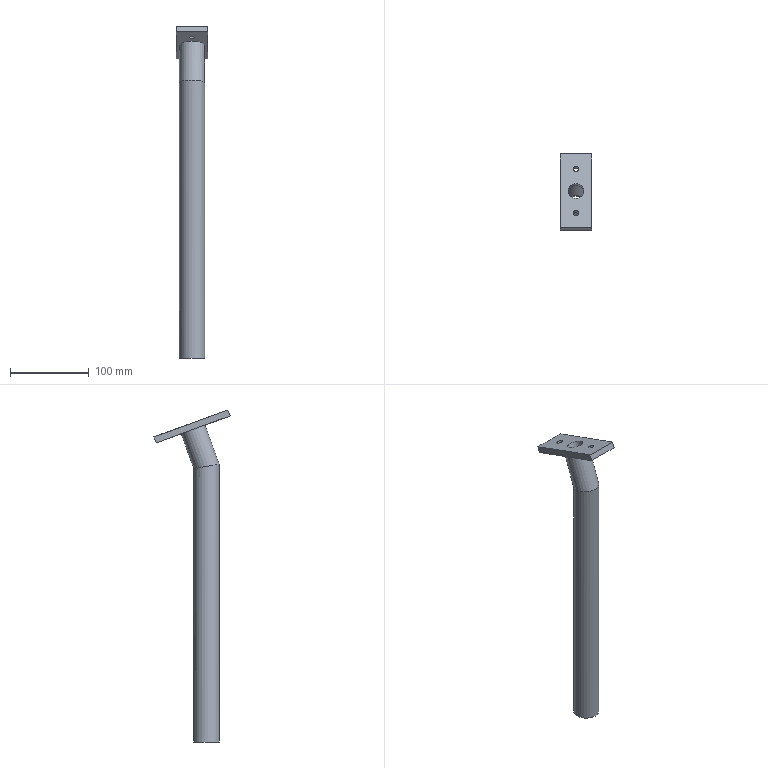Part | STEP file | 1112 | 1 solid | 15 faces | box 40 x 96.705 x 421.603 mm | volume 104269 mm3 | plane 8 | cylinder 7 | commonest cylinder face diameters 7 x2 28 x2 32 x2 20 x1
STEP:
#1=CARTESIAN_POINT('',(0.,0.,0.));
#2=DIRECTION('',(0.,0.,1.));
#3=DIRECTION('',(1.,0.,0.));
#4=AXIS2_PLACEMENT_3D('',#1,#2,#3);
#5=CARTESIAN_POINT('',(0.,-20.316,30.363));
#6=VERTEX_POINT('',#5);
#7=CARTESIAN_POINT('',(0.,11.684,24.721));
#8=VERTEX_POINT('',#7);
#9=CARTESIAN_POINT('',(0.,11.684,24.721));
#10=CARTESIAN_POINT('',(32.,11.684,24.721));
#11=CARTESIAN_POINT('',(32.,-20.316,30.363));
#12=CARTESIAN_POINT('',(0.,-20.316,30.363));
#13=CARTESIAN_POINT('',(-32.,-20.316,30.363));
#14=CARTESIAN_POINT('',(-32.,11.684,24.721));
#15=CARTESIAN_POINT('',(0.,11.684,24.721));
#16=(BOUNDED_CURVE()B_SPLINE_CURVE(3,(#9,#10,#11,#12,#13,#14,#15),.UNSPECIFIED.,.T.,.F.)B_SPLINE_CURVE_WITH_KNOTS((1,3,3,3,1),(-3.142,0.,3.142,6.283,9.425),.UNSPECIFIED.)CURVE()GEOMETRIC_REPRESENTATION_ITEM()RATIONAL_B_SPLINE_CURVE((1.,0.3333,0.3333,1.,0.3333,0.3333,1.))REPRESENTATION_ITEM(''));
#17=CARTESIAN_POINT('',(0.,-4.316,27.542));
#18=DIRECTION('',(0.,0.342,0.9397));
#19=DIRECTION('',(0.,-0.9397,0.342));
#20=AXIS2_PLACEMENT_3D('',#17,#18,#19);
#21=CYLINDRICAL_SURFACE('',#20,16.);
#22=CARTESIAN_POINT('',(9.425,2.821));
#23=CARTESIAN_POINT('',(9.364,2.821));
#24=CARTESIAN_POINT('',(9.232,2.791));
#25=CARTESIAN_POINT('',(8.995,2.593));
#26=CARTESIAN_POINT('',(8.714,2.172));
#27=CARTESIAN_POINT('',(8.392,1.474));
#28=CARTESIAN_POINT('',(8.037,0.5262));
#29=CARTESIAN_POINT('',(7.671,-0.5261));
#30=CARTESIAN_POINT('',(7.316,-1.474));
#31=CARTESIAN_POINT('',(6.994,-2.172));
#32=CARTESIAN_POINT('',(6.714,-2.593));
#33=CARTESIAN_POINT('',(6.475,-2.791));
#34=CARTESIAN_POINT('',(6.283,-2.837));
#35=CARTESIAN_POINT('',(6.092,-2.791));
#36=CARTESIAN_POINT('',(5.853,-2.593));
#37=CARTESIAN_POINT('',(5.573,-2.172));
#38=CARTESIAN_POINT('',(5.25,-1.474));
#39=CARTESIAN_POINT('',(4.896,-0.5261));
#40=CARTESIAN_POINT('',(4.529,0.5262));
#41=CARTESIAN_POINT('',(4.175,1.474));
#42=CARTESIAN_POINT('',(3.852,2.172));
#43=CARTESIAN_POINT('',(3.572,2.593));
#44=CARTESIAN_POINT('',(3.335,2.791));
#45=CARTESIAN_POINT('',(3.202,2.821));
#46=CARTESIAN_POINT('',(3.142,2.821));
#47=B_SPLINE_CURVE_WITH_KNOTS('',3,(#22,#23,#24,#25,#26,#27,#28,#29,#30,#31,#32,#33,#34,#35,#36,#37,#38,#39,#40,#41,#42,#43,#44,#45,#46),.UNSPECIFIED.,.F.,.F.,(4,1,1,1,1,1,1,1,1,1,1,1,1,1,1,1,1,1,1,1,1,1,4),(0.,0.2856,0.5712,0.8568,1.142,1.428,1.714,1.999,2.285,2.57,2.856,3.142,3.427,3.713,3.998,4.284,4.57,4.855,5.141,5.426,5.712,5.998,6.283),.QUASI_UNIFORM_KNOTS.);
#48=(GEOMETRIC_REPRESENTATION_CONTEXT(2)PARAMETRIC_REPRESENTATION_CONTEXT()REPRESENTATION_CONTEXT('',''));
#49=DEFINITIONAL_REPRESENTATION('',(#47),#48);
#50=PCURVE('',#21,#49);
#51=CARTESIAN_POINT('',(0.,-4.316,72.797));
#52=DIRECTION('',(0.,0.,-1.));
#53=DIRECTION('',(0.,1.,0.));
#54=AXIS2_PLACEMENT_3D('',#51,#52,#53);
#55=CYLINDRICAL_SURFACE('',#54,16.);
#56=CARTESIAN_POINT('',(3.142,42.434));
#57=CARTESIAN_POINT('',(3.172,42.434));
#58=CARTESIAN_POINT('',(3.235,42.441));
#59=CARTESIAN_POINT('',(3.339,42.483));
#60=CARTESIAN_POINT('',(3.453,42.563));
#61=CARTESIAN_POINT('',(3.577,42.69));
#62=CARTESIAN_POINT('',(3.712,42.872));
#63=CARTESIAN_POINT('',(3.857,43.118));
#64=CARTESIAN_POINT('',(4.013,43.431));
#65=CARTESIAN_POINT('',(4.179,43.812));
#66=CARTESIAN_POINT('',(4.352,44.254));
#67=CARTESIAN_POINT('',(4.531,44.742));
#68=CARTESIAN_POINT('',(4.712,45.255));
#69=CARTESIAN_POINT('',(4.894,45.768));
#70=CARTESIAN_POINT('',(5.073,46.256));
#71=CARTESIAN_POINT('',(5.246,46.697));
#72=CARTESIAN_POINT('',(5.412,47.078));
#73=CARTESIAN_POINT('',(5.567,47.392));
#74=CARTESIAN_POINT('',(5.713,47.637));
#75=CARTESIAN_POINT('',(5.848,47.82));
#76=CARTESIAN_POINT('',(5.972,47.947));
#77=CARTESIAN_POINT('',(6.085,48.027));
#78=CARTESIAN_POINT('',(6.19,48.068));
#79=CARTESIAN_POINT('',(6.253,48.076));
#80=CARTESIAN_POINT('',(6.283,48.076));
#81=B_SPLINE_CURVE_WITH_KNOTS('',3,(#56,#57,#58,#59,#60,#61,#62,#63,#64,#65,#66,#67,#68,#69,#70,#71,#72,#73,#74,#75,#76,#77,#78,#79,#80),.UNSPECIFIED.,.F.,.F.,(4,1,1,1,1,1,1,1,1,1,1,1,1,1,1,1,1,1,1,1,1,1,4),(3.142,3.284,3.427,3.57,3.713,3.856,3.998,4.141,4.284,4.427,4.57,4.712,4.855,4.998,5.141,5.284,5.426,5.569,5.712,5.855,5.998,6.14,6.283),.QUASI_UNIFORM_KNOTS.);
#82=(GEOMETRIC_REPRESENTATION_CONTEXT(2)PARAMETRIC_REPRESENTATION_CONTEXT()REPRESENTATION_CONTEXT('',''));
#83=DEFINITIONAL_REPRESENTATION('',(#81),#82);
#84=PCURVE('',#55,#83);
#85=SURFACE_CURVE('',#16,(#50,#84),.PCURVE_S1.);
#86=EDGE_CURVE('',#6,#8,#85,.T.);
#87=ORIENTED_EDGE('',*,*,#86,.F.);
#88=CARTESIAN_POINT('',(0.,-2.25,79.999));
#89=VERTEX_POINT('',#88);
#90=CARTESIAN_POINT('',(0.,-20.316,30.363));
#91=CARTESIAN_POINT('',(0.,-2.25,79.999));
#92=B_SPLINE_CURVE_WITH_KNOTS('',1,(#90,#91),.UNSPECIFIED.,.F.,.F.,(2,2),(-2.821,50.),.PIECEWISE_BEZIER_KNOTS.);
#93=CARTESIAN_POINT('',(6.283,0.));
#94=DIRECTION('',(0.,1.));
#95=VECTOR('',#94,1.);
#96=LINE('',#93,#95);
#97=(GEOMETRIC_REPRESENTATION_CONTEXT(2)PARAMETRIC_REPRESENTATION_CONTEXT()REPRESENTATION_CONTEXT('',''));
#98=DEFINITIONAL_REPRESENTATION('',(#96),#97);
#99=PCURVE('',#21,#98);
#100=CARTESIAN_POINT('',(0.,0.));
#101=DIRECTION('',(0.,1.));
#102=VECTOR('',#101,1.);
#103=LINE('',#100,#102);
#104=(GEOMETRIC_REPRESENTATION_CONTEXT(2)PARAMETRIC_REPRESENTATION_CONTEXT()REPRESENTATION_CONTEXT('',''));
#105=DEFINITIONAL_REPRESENTATION('',(#103),#104);
#106=PCURVE('',#21,#105);
#107=SEAM_CURVE('',#92,(#99,#106),.PCURVE_S1.);
#108=EDGE_CURVE('',#6,#89,#107,.T.);
#109=ORIENTED_EDGE('',*,*,#108,.T.);
#110=CARTESIAN_POINT('',(0.,12.785,74.527));
#111=DIRECTION('',(0.,0.342,0.9397));
#112=DIRECTION('',(0.,-0.9397,0.342));
#113=AXIS2_PLACEMENT_3D('',#110,#111,#112);
#114=CIRCLE('',#113,16.);
#115=CARTESIAN_POINT('',(0.,50.));
#116=DIRECTION('',(1.,0.));
#117=VECTOR('',#116,1.);
#118=LINE('',#115,#117);
#119=(GEOMETRIC_REPRESENTATION_CONTEXT(2)PARAMETRIC_REPRESENTATION_CONTEXT()REPRESENTATION_CONTEXT('',''));
#120=DEFINITIONAL_REPRESENTATION('',(#118),#119);
#121=PCURVE('',#21,#120);
#122=CARTESIAN_POINT('',(0.,25.448,69.918));
#123=DIRECTION('',(0.,0.342,0.9397));
#124=DIRECTION('',(0.,-0.9397,0.342));
#125=AXIS2_PLACEMENT_3D('',#122,#123,#124);
#126=PLANE('',#125);
#127=CARTESIAN_POINT('',(13.476,0.));
#128=DIRECTION('',(1.,0.));
#129=AXIS2_PLACEMENT_2D('',#127,#128);
#130=CIRCLE('',#129,16.);
#131=(GEOMETRIC_REPRESENTATION_CONTEXT(2)PARAMETRIC_REPRESENTATION_CONTEXT()REPRESENTATION_CONTEXT('',''));
#132=DEFINITIONAL_REPRESENTATION('',(#130),#131);
#133=PCURVE('',#126,#132);
#134=SURFACE_CURVE('',#114,(#121,#133),.PCURVE_S1.);
#135=EDGE_CURVE('',#89,#89,#134,.T.);
#136=ORIENTED_EDGE('',*,*,#135,.F.);
#137=ORIENTED_EDGE('',*,*,#108,.F.);
#138=CARTESIAN_POINT('',(0.,11.684,24.721));
#139=CARTESIAN_POINT('',(32.,11.684,24.721));
#140=CARTESIAN_POINT('',(32.,-20.316,30.363));
#141=CARTESIAN_POINT('',(0.,-20.316,30.363));
#142=CARTESIAN_POINT('',(-32.,-20.316,30.363));
#143=CARTESIAN_POINT('',(-32.,11.684,24.721));
#144=CARTESIAN_POINT('',(0.,11.684,24.721));
#145=(BOUNDED_CURVE()B_SPLINE_CURVE(3,(#138,#139,#140,#141,#142,#143,#144),.UNSPECIFIED.,.T.,.F.)B_SPLINE_CURVE_WITH_KNOTS((1,3,3,3,1),(-3.142,0.,3.142,6.283,9.425),.UNSPECIFIED.)CURVE()GEOMETRIC_REPRESENTATION_ITEM()RATIONAL_B_SPLINE_CURVE((1.,0.3333,0.3333,1.,0.3333,0.3333,1.))REPRESENTATION_ITEM(''));
#146=CARTESIAN_POINT('',(3.142,2.821));
#147=CARTESIAN_POINT('',(3.081,2.821));
#148=CARTESIAN_POINT('',(2.949,2.791));
#149=CARTESIAN_POINT('',(2.711,2.593));
#150=CARTESIAN_POINT('',(2.431,2.172));
#151=CARTESIAN_POINT('',(2.109,1.474));
#152=CARTESIAN_POINT('',(1.754,0.5262));
#153=CARTESIAN_POINT('',(1.387,-0.5261));
#154=CARTESIAN_POINT('',(1.033,-1.474));
#155=CARTESIAN_POINT('',(0.7104,-2.172));
#156=CARTESIAN_POINT('',(0.4306,-2.593));
#157=CARTESIAN_POINT('',(0.1914,-2.791));
#158=CARTESIAN_POINT('',(0.,-2.837));
#159=CARTESIAN_POINT('',(-0.1914,-2.791));
#160=CARTESIAN_POINT('',(-0.4306,-2.593));
#161=CARTESIAN_POINT('',(-0.7104,-2.172));
#162=CARTESIAN_POINT('',(-1.033,-1.474));
#163=CARTESIAN_POINT('',(-1.387,-0.5261));
#164=CARTESIAN_POINT('',(-1.754,0.5262));
#165=CARTESIAN_POINT('',(-2.109,1.474));
#166=CARTESIAN_POINT('',(-2.431,2.172));
#167=CARTESIAN_POINT('',(-2.711,2.593));
#168=CARTESIAN_POINT('',(-2.949,2.791));
#169=CARTESIAN_POINT('',(-3.081,2.821));
#170=CARTESIAN_POINT('',(-3.142,2.821));
#171=B_SPLINE_CURVE_WITH_KNOTS('',3,(#146,#147,#148,#149,#150,#151,#152,#153,#154,#155,#156,#157,#158,#159,#160,#161,#162,#163,#164,#165,#166,#167,#168,#169,#170),.UNSPECIFIED.,.F.,.F.,(4,1,1,1,1,1,1,1,1,1,1,1,1,1,1,1,1,1,1,1,1,1,4),(0.,0.2856,0.5712,0.8568,1.142,1.428,1.714,1.999,2.285,2.57,2.856,3.142,3.427,3.713,3.998,4.284,4.57,4.855,5.141,5.426,5.712,5.998,6.283),.QUASI_UNIFORM_KNOTS.);
#172=(GEOMETRIC_REPRESENTATION_CONTEXT(2)PARAMETRIC_REPRESENTATION_CONTEXT()REPRESENTATION_CONTEXT('',''));
#173=DEFINITIONAL_REPRESENTATION('',(#171),#172);
#174=PCURVE('',#21,#173);
#175=CARTESIAN_POINT('',(0.,48.076));
#176=CARTESIAN_POINT('',(0.0303,48.076));
#177=CARTESIAN_POINT('',(0.09367,48.068));
#178=CARTESIAN_POINT('',(0.1977,48.027));
#179=CARTESIAN_POINT('',(0.3115,47.947));
#180=CARTESIAN_POINT('',(0.4356,47.82));
#181=CARTESIAN_POINT('',(0.5703,47.637));
#182=CARTESIAN_POINT('',(0.7158,47.392));
#183=CARTESIAN_POINT('',(0.8717,47.078));
#184=CARTESIAN_POINT('',(1.037,46.697));
#185=CARTESIAN_POINT('',(1.21,46.256));
#186=CARTESIAN_POINT('',(1.389,45.768));
#187=CARTESIAN_POINT('',(1.571,45.255));
#188=CARTESIAN_POINT('',(1.753,44.742));
#189=CARTESIAN_POINT('',(1.931,44.254));
#190=CARTESIAN_POINT('',(2.105,43.812));
#191=CARTESIAN_POINT('',(2.27,43.431));
#192=CARTESIAN_POINT('',(2.426,43.118));
#193=CARTESIAN_POINT('',(2.571,42.872));
#194=CARTESIAN_POINT('',(2.706,42.69));
#195=CARTESIAN_POINT('',(2.83,42.563));
#196=CARTESIAN_POINT('',(2.944,42.483));
#197=CARTESIAN_POINT('',(3.048,42.441));
#198=CARTESIAN_POINT('',(3.111,42.434));
#199=CARTESIAN_POINT('',(3.142,42.434));
#200=B_SPLINE_CURVE_WITH_KNOTS('',3,(#175,#176,#177,#178,#179,#180,#181,#182,#183,#184,#185,#186,#187,#188,#189,#190,#191,#192,#193,#194,#195,#196,#197,#198,#199),.UNSPECIFIED.,.F.,.F.,(4,1,1,1,1,1,1,1,1,1,1,1,1,1,1,1,1,1,1,1,1,1,4),(0.,0.1428,0.2856,0.4284,0.5712,0.714,0.8568,0.9996,1.142,1.285,1.428,1.571,1.714,1.856,1.999,2.142,2.285,2.428,2.57,2.713,2.856,2.999,3.142),.QUASI_UNIFORM_KNOTS.);
#201=(GEOMETRIC_REPRESENTATION_CONTEXT(2)PARAMETRIC_REPRESENTATION_CONTEXT()REPRESENTATION_CONTEXT('',''));
#202=DEFINITIONAL_REPRESENTATION('',(#200),#201);
#203=PCURVE('',#55,#202);
#204=SURFACE_CURVE('',#145,(#174,#203),.PCURVE_S1.);
#205=EDGE_CURVE('',#8,#6,#204,.T.);
#206=ORIENTED_EDGE('',*,*,#205,.F.);
#207=EDGE_LOOP('',(#87,#109,#136,#137,#206));
#208=FACE_BOUND('',#207,.T.);
#209=ADVANCED_FACE('',(#208),#21,.T.);
#210=CARTESIAN_POINT('',(0.,-18.316,30.011));
#211=VERTEX_POINT('',#210);
#212=CARTESIAN_POINT('',(0.,9.684,25.074));
#213=VERTEX_POINT('',#212);
#214=CARTESIAN_POINT('',(0.,9.684,25.074));
#215=CARTESIAN_POINT('',(28.,9.684,25.074));
#216=CARTESIAN_POINT('',(28.,-18.316,30.011));
#217=CARTESIAN_POINT('',(0.,-18.316,30.011));
#218=CARTESIAN_POINT('',(-28.,-18.316,30.011));
#219=CARTESIAN_POINT('',(-28.,9.684,25.074));
#220=CARTESIAN_POINT('',(0.,9.684,25.074));
#221=(BOUNDED_CURVE()B_SPLINE_CURVE(3,(#214,#215,#216,#217,#218,#219,#220),.UNSPECIFIED.,.T.,.F.)B_SPLINE_CURVE_WITH_KNOTS((1,3,3,3,1),(-3.142,0.,3.142,6.283,9.425),.UNSPECIFIED.)CURVE()GEOMETRIC_REPRESENTATION_ITEM()RATIONAL_B_SPLINE_CURVE((1.,0.3333,0.3333,1.,0.3333,0.3333,1.))REPRESENTATION_ITEM(''));
#222=CARTESIAN_POINT('',(0.,-4.316,27.542));
#223=DIRECTION('',(0.,0.342,0.9397));
#224=DIRECTION('',(0.,-0.9397,0.342));
#225=AXIS2_PLACEMENT_3D('',#222,#223,#224);
#226=CYLINDRICAL_SURFACE('',#225,14.);
#227=CARTESIAN_POINT('',(9.425,2.469));
#228=CARTESIAN_POINT('',(9.364,2.468));
#229=CARTESIAN_POINT('',(9.232,2.442));
#230=CARTESIAN_POINT('',(8.995,2.269));
#231=CARTESIAN_POINT('',(8.714,1.9));
#232=CARTESIAN_POINT('',(8.392,1.29));
#233=CARTESIAN_POINT('',(8.037,0.4604));
#234=CARTESIAN_POINT('',(7.671,-0.4604));
#235=CARTESIAN_POINT('',(7.316,-1.29));
#236=CARTESIAN_POINT('',(6.994,-1.9));
#237=CARTESIAN_POINT('',(6.714,-2.269));
#238=CARTESIAN_POINT('',(6.475,-2.442));
#239=CARTESIAN_POINT('',(6.283,-2.482));
#240=CARTESIAN_POINT('',(6.092,-2.442));
#241=CARTESIAN_POINT('',(5.853,-2.269));
#242=CARTESIAN_POINT('',(5.573,-1.9));
#243=CARTESIAN_POINT('',(5.25,-1.29));
#244=CARTESIAN_POINT('',(4.896,-0.4604));
#245=CARTESIAN_POINT('',(4.529,0.4604));
#246=CARTESIAN_POINT('',(4.175,1.29));
#247=CARTESIAN_POINT('',(3.852,1.9));
#248=CARTESIAN_POINT('',(3.572,2.269));
#249=CARTESIAN_POINT('',(3.335,2.442));
#250=CARTESIAN_POINT('',(3.202,2.468));
#251=CARTESIAN_POINT('',(3.142,2.469));
#252=B_SPLINE_CURVE_WITH_KNOTS('',3,(#227,#228,#229,#230,#231,#232,#233,#234,#235,#236,#237,#238,#239,#240,#241,#242,#243,#244,#245,#246,#247,#248,#249,#250,#251),.UNSPECIFIED.,.F.,.F.,(4,1,1,1,1,1,1,1,1,1,1,1,1,1,1,1,1,1,1,1,1,1,4),(0.,0.2856,0.5712,0.8568,1.142,1.428,1.714,1.999,2.285,2.57,2.856,3.142,3.427,3.713,3.998,4.284,4.57,4.855,5.141,5.426,5.712,5.998,6.283),.QUASI_UNIFORM_KNOTS.);
#253=(GEOMETRIC_REPRESENTATION_CONTEXT(2)PARAMETRIC_REPRESENTATION_CONTEXT()REPRESENTATION_CONTEXT('',''));
#254=DEFINITIONAL_REPRESENTATION('',(#252),#253);
#255=PCURVE('',#226,#254);
#256=CARTESIAN_POINT('',(0.,-4.316,72.797));
#257=DIRECTION('',(0.,0.,-1.));
#258=DIRECTION('',(0.,1.,0.));
#259=AXIS2_PLACEMENT_3D('',#256,#257,#258);
#260=CYLINDRICAL_SURFACE('',#259,14.);
#261=CARTESIAN_POINT('',(3.142,42.786));
#262=CARTESIAN_POINT('',(3.172,42.786));
#263=CARTESIAN_POINT('',(3.235,42.793));
#264=CARTESIAN_POINT('',(3.339,42.83));
#265=CARTESIAN_POINT('',(3.453,42.9));
#266=CARTESIAN_POINT('',(3.577,43.01));
#267=CARTESIAN_POINT('',(3.712,43.17));
#268=CARTESIAN_POINT('',(3.857,43.385));
#269=CARTESIAN_POINT('',(4.013,43.659));
#270=CARTESIAN_POINT('',(4.179,43.993));
#271=CARTESIAN_POINT('',(4.352,44.379));
#272=CARTESIAN_POINT('',(4.531,44.806));
#273=CARTESIAN_POINT('',(4.712,45.255));
#274=CARTESIAN_POINT('',(4.894,45.704));
#275=CARTESIAN_POINT('',(5.073,46.131));
#276=CARTESIAN_POINT('',(5.246,46.517));
#277=CARTESIAN_POINT('',(5.412,46.85));
#278=CARTESIAN_POINT('',(5.567,47.125));
#279=CARTESIAN_POINT('',(5.713,47.34));
#280=CARTESIAN_POINT('',(5.848,47.499));
#281=CARTESIAN_POINT('',(5.972,47.61));
#282=CARTESIAN_POINT('',(6.085,47.68));
#283=CARTESIAN_POINT('',(6.19,47.717));
#284=CARTESIAN_POINT('',(6.253,47.723));
#285=CARTESIAN_POINT('',(6.283,47.723));
#286=B_SPLINE_CURVE_WITH_KNOTS('',3,(#261,#262,#263,#264,#265,#266,#267,#268,#269,#270,#271,#272,#273,#274,#275,#276,#277,#278,#279,#280,#281,#282,#283,#284,#285),.UNSPECIFIED.,.F.,.F.,(4,1,1,1,1,1,1,1,1,1,1,1,1,1,1,1,1,1,1,1,1,1,4),(3.142,3.284,3.427,3.57,3.713,3.856,3.998,4.141,4.284,4.427,4.57,4.712,4.855,4.998,5.141,5.284,5.426,5.569,5.712,5.855,5.998,6.14,6.283),.QUASI_UNIFORM_KNOTS.);
#287=(GEOMETRIC_REPRESENTATION_CONTEXT(2)PARAMETRIC_REPRESENTATION_CONTEXT()REPRESENTATION_CONTEXT('',''));
#288=DEFINITIONAL_REPRESENTATION('',(#286),#287);
#289=PCURVE('',#260,#288);
#290=SURFACE_CURVE('',#221,(#255,#289),.PCURVE_S1.);
#291=EDGE_CURVE('',#211,#213,#290,.T.);
#292=ORIENTED_EDGE('',*,*,#291,.F.);
#293=CARTESIAN_POINT('',(0.,-0.371,79.315));
#294=VERTEX_POINT('',#293);
#295=CARTESIAN_POINT('',(0.,-18.316,30.011));
#296=CARTESIAN_POINT('',(0.,-0.371,79.315));
#297=B_SPLINE_CURVE_WITH_KNOTS('',1,(#295,#296),.UNSPECIFIED.,.F.,.F.,(2,2),(-2.469,50.),.PIECEWISE_BEZIER_KNOTS.);
#298=CARTESIAN_POINT('',(6.283,0.));
#299=DIRECTION('',(0.,1.));
#300=VECTOR('',#299,1.);
#301=LINE('',#298,#300);
#302=(GEOMETRIC_REPRESENTATION_CONTEXT(2)PARAMETRIC_REPRESENTATION_CONTEXT()REPRESENTATION_CONTEXT('',''));
#303=DEFINITIONAL_REPRESENTATION('',(#301),#302);
#304=PCURVE('',#226,#303);
#305=CARTESIAN_POINT('',(0.,0.));
#306=DIRECTION('',(0.,1.));
#307=VECTOR('',#306,1.);
#308=LINE('',#305,#307);
#309=(GEOMETRIC_REPRESENTATION_CONTEXT(2)PARAMETRIC_REPRESENTATION_CONTEXT()REPRESENTATION_CONTEXT('',''));
#310=DEFINITIONAL_REPRESENTATION('',(#308),#309);
#311=PCURVE('',#226,#310);
#312=SEAM_CURVE('',#297,(#304,#311),.PCURVE_S1.);
#313=EDGE_CURVE('',#211,#294,#312,.T.);
#314=ORIENTED_EDGE('',*,*,#313,.T.);
#315=CARTESIAN_POINT('',(0.,12.785,74.527));
#316=DIRECTION('',(0.,0.342,0.9397));
#317=DIRECTION('',(0.,-0.9397,0.342));
#318=AXIS2_PLACEMENT_3D('',#315,#316,#317);
#319=CIRCLE('',#318,14.);
#320=CARTESIAN_POINT('',(0.,50.));
#321=DIRECTION('',(1.,0.));
#322=VECTOR('',#321,1.);
#323=LINE('',#320,#322);
#324=(GEOMETRIC_REPRESENTATION_CONTEXT(2)PARAMETRIC_REPRESENTATION_CONTEXT()REPRESENTATION_CONTEXT('',''));
#325=DEFINITIONAL_REPRESENTATION('',(#323),#324);
#326=PCURVE('',#226,#325);
#327=CARTESIAN_POINT('',(0.,25.448,69.918));
#328=DIRECTION('',(0.,0.342,0.9397));
#329=DIRECTION('',(0.,-0.9397,0.342));
#330=AXIS2_PLACEMENT_3D('',#327,#328,#329);
#331=PLANE('',#330);
#332=CARTESIAN_POINT('',(13.476,0.));
#333=DIRECTION('',(1.,0.));
#334=AXIS2_PLACEMENT_2D('',#332,#333);
#335=CIRCLE('',#334,14.);
#336=(GEOMETRIC_REPRESENTATION_CONTEXT(2)PARAMETRIC_REPRESENTATION_CONTEXT()REPRESENTATION_CONTEXT('',''));
#337=DEFINITIONAL_REPRESENTATION('',(#335),#336);
#338=PCURVE('',#331,#337);
#339=SURFACE_CURVE('',#319,(#326,#338),.PCURVE_S1.);
#340=EDGE_CURVE('',#294,#294,#339,.T.);
#341=ORIENTED_EDGE('',*,*,#340,.F.);
#342=ORIENTED_EDGE('',*,*,#313,.F.);
#343=CARTESIAN_POINT('',(0.,9.684,25.074));
#344=CARTESIAN_POINT('',(28.,9.684,25.074));
#345=CARTESIAN_POINT('',(28.,-18.316,30.011));
#346=CARTESIAN_POINT('',(0.,-18.316,30.011));
#347=CARTESIAN_POINT('',(-28.,-18.316,30.011));
#348=CARTESIAN_POINT('',(-28.,9.684,25.074));
#349=CARTESIAN_POINT('',(0.,9.684,25.074));
#350=(BOUNDED_CURVE()B_SPLINE_CURVE(3,(#343,#344,#345,#346,#347,#348,#349),.UNSPECIFIED.,.T.,.F.)B_SPLINE_CURVE_WITH_KNOTS((1,3,3,3,1),(-3.142,0.,3.142,6.283,9.425),.UNSPECIFIED.)CURVE()GEOMETRIC_REPRESENTATION_ITEM()RATIONAL_B_SPLINE_CURVE((1.,0.3333,0.3333,1.,0.3333,0.3333,1.))REPRESENTATION_ITEM(''));
#351=CARTESIAN_POINT('',(3.142,2.469));
#352=CARTESIAN_POINT('',(3.081,2.468));
#353=CARTESIAN_POINT('',(2.949,2.442));
#354=CARTESIAN_POINT('',(2.711,2.269));
#355=CARTESIAN_POINT('',(2.431,1.9));
#356=CARTESIAN_POINT('',(2.109,1.29));
#357=CARTESIAN_POINT('',(1.754,0.4604));
#358=CARTESIAN_POINT('',(1.387,-0.4604));
#359=CARTESIAN_POINT('',(1.033,-1.29));
#360=CARTESIAN_POINT('',(0.7104,-1.9));
#361=CARTESIAN_POINT('',(0.4306,-2.269));
#362=CARTESIAN_POINT('',(0.1914,-2.442));
#363=CARTESIAN_POINT('',(0.,-2.482));
#364=CARTESIAN_POINT('',(-0.1914,-2.442));
#365=CARTESIAN_POINT('',(-0.4306,-2.269));
#366=CARTESIAN_POINT('',(-0.7104,-1.9));
#367=CARTESIAN_POINT('',(-1.033,-1.29));
#368=CARTESIAN_POINT('',(-1.387,-0.4604));
#369=CARTESIAN_POINT('',(-1.754,0.4604));
#370=CARTESIAN_POINT('',(-2.109,1.29));
#371=CARTESIAN_POINT('',(-2.431,1.9));
#372=CARTESIAN_POINT('',(-2.711,2.269));
#373=CARTESIAN_POINT('',(-2.949,2.442));
#374=CARTESIAN_POINT('',(-3.081,2.468));
#375=CARTESIAN_POINT('',(-3.142,2.469));
#376=B_SPLINE_CURVE_WITH_KNOTS('',3,(#351,#352,#353,#354,#355,#356,#357,#358,#359,#360,#361,#362,#363,#364,#365,#366,#367,#368,#369,#370,#371,#372,#373,#374,#375),.UNSPECIFIED.,.F.,.F.,(4,1,1,1,1,1,1,1,1,1,1,1,1,1,1,1,1,1,1,1,1,1,4),(0.,0.2856,0.5712,0.8568,1.142,1.428,1.714,1.999,2.285,2.57,2.856,3.142,3.427,3.713,3.998,4.284,4.57,4.855,5.141,5.426,5.712,5.998,6.283),.QUASI_UNIFORM_KNOTS.);
#377=(GEOMETRIC_REPRESENTATION_CONTEXT(2)PARAMETRIC_REPRESENTATION_CONTEXT()REPRESENTATION_CONTEXT('',''));
#378=DEFINITIONAL_REPRESENTATION('',(#376),#377);
#379=PCURVE('',#226,#378);
#380=CARTESIAN_POINT('',(0.,47.723));
#381=CARTESIAN_POINT('',(0.0303,47.723));
#382=CARTESIAN_POINT('',(0.09367,47.717));
#383=CARTESIAN_POINT('',(0.1977,47.68));
#384=CARTESIAN_POINT('',(0.3115,47.61));
#385=CARTESIAN_POINT('',(0.4356,47.499));
#386=CARTESIAN_POINT('',(0.5703,47.34));
#387=CARTESIAN_POINT('',(0.7158,47.125));
#388=CARTESIAN_POINT('',(0.8717,46.85));
#389=CARTESIAN_POINT('',(1.037,46.517));
#390=CARTESIAN_POINT('',(1.21,46.131));
#391=CARTESIAN_POINT('',(1.389,45.704));
#392=CARTESIAN_POINT('',(1.571,45.255));
#393=CARTESIAN_POINT('',(1.753,44.806));
#394=CARTESIAN_POINT('',(1.931,44.379));
#395=CARTESIAN_POINT('',(2.105,43.993));
#396=CARTESIAN_POINT('',(2.27,43.659));
#397=CARTESIAN_POINT('',(2.426,43.385));
#398=CARTESIAN_POINT('',(2.571,43.17));
#399=CARTESIAN_POINT('',(2.706,43.01));
#400=CARTESIAN_POINT('',(2.83,42.9));
#401=CARTESIAN_POINT('',(2.944,42.83));
#402=CARTESIAN_POINT('',(3.048,42.793));
#403=CARTESIAN_POINT('',(3.111,42.786));
#404=CARTESIAN_POINT('',(3.142,42.786));
#405=B_SPLINE_CURVE_WITH_KNOTS('',3,(#380,#381,#382,#383,#384,#385,#386,#387,#388,#389,#390,#391,#392,#393,#394,#395,#396,#397,#398,#399,#400,#401,#402,#403,#404),.UNSPECIFIED.,.F.,.F.,(4,1,1,1,1,1,1,1,1,1,1,1,1,1,1,1,1,1,1,1,1,1,4),(0.,0.1428,0.2856,0.4284,0.5712,0.714,0.8568,0.9996,1.142,1.285,1.428,1.571,1.714,1.856,1.999,2.142,2.285,2.428,2.57,2.713,2.856,2.999,3.142),.QUASI_UNIFORM_KNOTS.);
#406=(GEOMETRIC_REPRESENTATION_CONTEXT(2)PARAMETRIC_REPRESENTATION_CONTEXT()REPRESENTATION_CONTEXT('',''));
#407=DEFINITIONAL_REPRESENTATION('',(#405),#406);
#408=PCURVE('',#260,#407);
#409=SURFACE_CURVE('',#350,(#379,#408),.PCURVE_S1.);
#410=EDGE_CURVE('',#213,#211,#409,.T.);
#411=ORIENTED_EDGE('',*,*,#410,.F.);
#412=EDGE_LOOP('',(#292,#314,#341,#342,#411));
#413=FACE_BOUND('',#412,.F.);
#414=ADVANCED_FACE('',(#413),#226,.F.);
#415=CARTESIAN_POINT('',(0.,9.684,-322.458));
#416=VERTEX_POINT('',#415);
#417=CARTESIAN_POINT('',(0.,-4.316,-322.458));
#418=DIRECTION('',(0.,0.,-1.));
#419=DIRECTION('',(0.,1.,0.));
#420=AXIS2_PLACEMENT_3D('',#417,#418,#419);
#421=CIRCLE('',#420,14.);
#422=CARTESIAN_POINT('',(0.,395.255));
#423=DIRECTION('',(1.,0.));
#424=VECTOR('',#423,1.);
#425=LINE('',#422,#424);
#426=(GEOMETRIC_REPRESENTATION_CONTEXT(2)PARAMETRIC_REPRESENTATION_CONTEXT()REPRESENTATION_CONTEXT('',''));
#427=DEFINITIONAL_REPRESENTATION('',(#425),#426);
#428=PCURVE('',#260,#427);
#429=CARTESIAN_POINT('',(0.,-4.316,-322.458));
#430=DIRECTION('',(0.,0.,-1.));
#431=DIRECTION('',(0.,1.,0.));
#432=AXIS2_PLACEMENT_3D('',#429,#430,#431);
#433=PLANE('',#432);
#434=CARTESIAN_POINT('',(0.,0.));
#435=DIRECTION('',(1.,0.));
#436=AXIS2_PLACEMENT_2D('',#434,#435);
#437=CIRCLE('',#436,14.);
#438=(GEOMETRIC_REPRESENTATION_CONTEXT(2)PARAMETRIC_REPRESENTATION_CONTEXT()REPRESENTATION_CONTEXT('',''));
#439=DEFINITIONAL_REPRESENTATION('',(#437),#438);
#440=PCURVE('',#433,#439);
#441=SURFACE_CURVE('',#421,(#428,#440),.PCURVE_S1.);
#442=EDGE_CURVE('',#416,#416,#441,.T.);
#443=ORIENTED_EDGE('',*,*,#442,.F.);
#444=CARTESIAN_POINT('',(0.,9.684,25.074));
#445=CARTESIAN_POINT('',(0.,9.684,-322.458));
#446=B_SPLINE_CURVE_WITH_KNOTS('',1,(#444,#445),.UNSPECIFIED.,.F.,.F.,(2,2),(47.723,395.255),.PIECEWISE_BEZIER_KNOTS.);
#447=CARTESIAN_POINT('',(0.,0.));
#448=DIRECTION('',(0.,1.));
#449=VECTOR('',#448,1.);
#450=LINE('',#447,#449);
#451=(GEOMETRIC_REPRESENTATION_CONTEXT(2)PARAMETRIC_REPRESENTATION_CONTEXT()REPRESENTATION_CONTEXT('',''));
#452=DEFINITIONAL_REPRESENTATION('',(#450),#451);
#453=PCURVE('',#260,#452);
#454=CARTESIAN_POINT('',(6.283,0.));
#455=DIRECTION('',(0.,1.));
#456=VECTOR('',#455,1.);
#457=LINE('',#454,#456);
#458=(GEOMETRIC_REPRESENTATION_CONTEXT(2)PARAMETRIC_REPRESENTATION_CONTEXT()REPRESENTATION_CONTEXT('',''));
#459=DEFINITIONAL_REPRESENTATION('',(#457),#458);
#460=PCURVE('',#260,#459);
#461=SEAM_CURVE('',#446,(#453,#460),.PCURVE_S1.);
#462=EDGE_CURVE('',#213,#416,#461,.T.);
#463=ORIENTED_EDGE('',*,*,#462,.F.);
#464=ORIENTED_EDGE('',*,*,#410,.T.);
#465=ORIENTED_EDGE('',*,*,#291,.T.);
#466=ORIENTED_EDGE('',*,*,#462,.T.);
#467=EDGE_LOOP('',(#443,#463,#464,#465,#466));
#468=FACE_BOUND('',#467,.F.);
#469=ADVANCED_FACE('',(#468),#260,.F.);
#470=ORIENTED_EDGE('',*,*,#442,.F.);
#471=EDGE_LOOP('',(#470));
#472=FACE_BOUND('',#471,.T.);
#473=CARTESIAN_POINT('',(0.,11.684,-322.458));
#474=VERTEX_POINT('',#473);
#475=CARTESIAN_POINT('',(0.,-4.316,-322.458));
#476=DIRECTION('',(0.,0.,-1.));
#477=DIRECTION('',(0.,1.,0.));
#478=AXIS2_PLACEMENT_3D('',#475,#476,#477);
#479=CIRCLE('',#478,16.);
#480=CARTESIAN_POINT('',(0.,0.));
#481=DIRECTION('',(1.,0.));
#482=AXIS2_PLACEMENT_2D('',#480,#481);
#483=CIRCLE('',#482,16.);
#484=(GEOMETRIC_REPRESENTATION_CONTEXT(2)PARAMETRIC_REPRESENTATION_CONTEXT()REPRESENTATION_CONTEXT('',''));
#485=DEFINITIONAL_REPRESENTATION('',(#483),#484);
#486=PCURVE('',#433,#485);
#487=CARTESIAN_POINT('',(0.,395.255));
#488=DIRECTION('',(1.,0.));
#489=VECTOR('',#488,1.);
#490=LINE('',#487,#489);
#491=(GEOMETRIC_REPRESENTATION_CONTEXT(2)PARAMETRIC_REPRESENTATION_CONTEXT()REPRESENTATION_CONTEXT('',''));
#492=DEFINITIONAL_REPRESENTATION('',(#490),#491);
#493=PCURVE('',#55,#492);
#494=SURFACE_CURVE('',#479,(#486,#493),.PCURVE_S1.);
#495=EDGE_CURVE('',#474,#474,#494,.T.);
#496=ORIENTED_EDGE('',*,*,#495,.T.);
#497=EDGE_LOOP('',(#496));
#498=FACE_BOUND('',#497,.T.);
#499=ADVANCED_FACE('',(#472,#498),#433,.T.);
#500=ORIENTED_EDGE('',*,*,#495,.F.);
#501=CARTESIAN_POINT('',(0.,11.684,24.721));
#502=CARTESIAN_POINT('',(0.,11.684,-322.458));
#503=B_SPLINE_CURVE_WITH_KNOTS('',1,(#501,#502),.UNSPECIFIED.,.F.,.F.,(2,2),(48.076,395.255),.PIECEWISE_BEZIER_KNOTS.);
#504=CARTESIAN_POINT('',(0.,0.));
#505=DIRECTION('',(0.,1.));
#506=VECTOR('',#505,1.);
#507=LINE('',#504,#506);
#508=(GEOMETRIC_REPRESENTATION_CONTEXT(2)PARAMETRIC_REPRESENTATION_CONTEXT()REPRESENTATION_CONTEXT('',''));
#509=DEFINITIONAL_REPRESENTATION('',(#507),#508);
#510=PCURVE('',#55,#509);
#511=CARTESIAN_POINT('',(6.283,0.));
#512=DIRECTION('',(0.,1.));
#513=VECTOR('',#512,1.);
#514=LINE('',#511,#513);
#515=(GEOMETRIC_REPRESENTATION_CONTEXT(2)PARAMETRIC_REPRESENTATION_CONTEXT()REPRESENTATION_CONTEXT('',''));
#516=DEFINITIONAL_REPRESENTATION('',(#514),#515);
#517=PCURVE('',#55,#516);
#518=SEAM_CURVE('',#503,(#510,#517),.PCURVE_S1.);
#519=EDGE_CURVE('',#8,#474,#518,.T.);
#520=ORIENTED_EDGE('',*,*,#519,.F.);
#521=ORIENTED_EDGE('',*,*,#205,.T.);
#522=ORIENTED_EDGE('',*,*,#86,.T.);
#523=ORIENTED_EDGE('',*,*,#519,.T.);
#524=EDGE_LOOP('',(#500,#520,#521,#522,#523));
#525=FACE_BOUND('',#524,.T.);
#526=ADVANCED_FACE('',(#525),#55,.T.);
#527=CARTESIAN_POINT('',(0.,3.388,77.947));
#528=VERTEX_POINT('',#527);
#529=CARTESIAN_POINT('',(0.,12.785,74.527));
#530=DIRECTION('',(0.,0.342,0.9397));
#531=DIRECTION('',(0.,-0.9397,0.342));
#532=AXIS2_PLACEMENT_3D('',#529,#530,#531);
#533=CIRCLE('',#532,10.);
#534=CARTESIAN_POINT('',(13.476,0.));
#535=DIRECTION('',(1.,0.));
#536=AXIS2_PLACEMENT_2D('',#534,#535);
#537=CIRCLE('',#536,10.);
#538=(GEOMETRIC_REPRESENTATION_CONTEXT(2)PARAMETRIC_REPRESENTATION_CONTEXT()REPRESENTATION_CONTEXT('',''));
#539=DEFINITIONAL_REPRESENTATION('',(#537),#538);
#540=PCURVE('',#331,#539);
#541=CARTESIAN_POINT('',(0.,12.785,74.527));
#542=DIRECTION('',(0.,0.342,0.9397));
#543=DIRECTION('',(0.,-0.9397,0.342));
#544=AXIS2_PLACEMENT_3D('',#541,#542,#543);
#545=CYLINDRICAL_SURFACE('',#544,10.);
#546=CARTESIAN_POINT('',(0.,0.));
#547=DIRECTION('',(1.,0.));
#548=VECTOR('',#547,1.);
#549=LINE('',#546,#548);
#550=(GEOMETRIC_REPRESENTATION_CONTEXT(2)PARAMETRIC_REPRESENTATION_CONTEXT()REPRESENTATION_CONTEXT('',''));
#551=DEFINITIONAL_REPRESENTATION('',(#549),#550);
#552=PCURVE('',#545,#551);
#553=SURFACE_CURVE('',#533,(#540,#552),.PCURVE_S1.);
#554=EDGE_CURVE('',#528,#528,#553,.T.);
#555=ORIENTED_EDGE('',*,*,#554,.T.);
#556=EDGE_LOOP('',(#555));
#557=FACE_BOUND('',#556,.T.);
#558=ORIENTED_EDGE('',*,*,#340,.F.);
#559=EDGE_LOOP('',(#558));
#560=FACE_BOUND('',#559,.T.);
#561=ADVANCED_FACE('',(#557,#560),#331,.F.);
#562=CARTESIAN_POINT('',(0.,-18.695,85.984));
#563=VERTEX_POINT('',#562);
#564=CARTESIAN_POINT('',(0.,-15.406,84.787));
#565=DIRECTION('',(0.,0.342,0.9397));
#566=DIRECTION('',(0.,-0.9397,0.342));
#567=AXIS2_PLACEMENT_3D('',#564,#565,#566);
#568=CIRCLE('',#567,3.5);
#569=CARTESIAN_POINT('',(43.476,0.));
#570=DIRECTION('',(1.,0.));
#571=AXIS2_PLACEMENT_2D('',#569,#570);
#572=CIRCLE('',#571,3.5);
#573=(GEOMETRIC_REPRESENTATION_CONTEXT(2)PARAMETRIC_REPRESENTATION_CONTEXT()REPRESENTATION_CONTEXT('',''));
#574=DEFINITIONAL_REPRESENTATION('',(#572),#573);
#575=PCURVE('',#126,#574);
#576=CARTESIAN_POINT('',(0.,-15.406,84.787));
#577=DIRECTION('',(0.,0.342,0.9397));
#578=DIRECTION('',(0.,-0.9397,0.342));
#579=AXIS2_PLACEMENT_3D('',#576,#577,#578);
#580=CYLINDRICAL_SURFACE('',#579,3.5);
#581=CARTESIAN_POINT('',(0.,0.));
#582=DIRECTION('',(1.,0.));
#583=VECTOR('',#582,1.);
#584=LINE('',#581,#583);
#585=(GEOMETRIC_REPRESENTATION_CONTEXT(2)PARAMETRIC_REPRESENTATION_CONTEXT()REPRESENTATION_CONTEXT('',''));
#586=DEFINITIONAL_REPRESENTATION('',(#584),#585);
#587=PCURVE('',#580,#586);
#588=SURFACE_CURVE('',#568,(#575,#587),.PCURVE_S1.);
#589=EDGE_CURVE('',#563,#563,#588,.T.);
#590=ORIENTED_EDGE('',*,*,#589,.T.);
#591=EDGE_LOOP('',(#590));
#592=FACE_BOUND('',#591,.T.);
#593=CARTESIAN_POINT('',(0.,37.687,65.463));
#594=VERTEX_POINT('',#593);
#595=CARTESIAN_POINT('',(0.,40.975,64.266));
#596=DIRECTION('',(0.,0.342,0.9397));
#597=DIRECTION('',(0.,-0.9397,0.342));
#598=AXIS2_PLACEMENT_3D('',#595,#596,#597);
#599=CIRCLE('',#598,3.5);
#600=CARTESIAN_POINT('',(-16.524,0.));
#601=DIRECTION('',(1.,0.));
#602=AXIS2_PLACEMENT_2D('',#600,#601);
#603=CIRCLE('',#602,3.5);
#604=(GEOMETRIC_REPRESENTATION_CONTEXT(2)PARAMETRIC_REPRESENTATION_CONTEXT()REPRESENTATION_CONTEXT('',''));
#605=DEFINITIONAL_REPRESENTATION('',(#603),#604);
#606=PCURVE('',#126,#605);
#607=CARTESIAN_POINT('',(0.,40.975,64.266));
#608=DIRECTION('',(0.,0.342,0.9397));
#609=DIRECTION('',(0.,-0.9397,0.342));
#610=AXIS2_PLACEMENT_3D('',#607,#608,#609);
#611=CYLINDRICAL_SURFACE('',#610,3.5);
#612=CARTESIAN_POINT('',(0.,0.));
#613=DIRECTION('',(1.,0.));
#614=VECTOR('',#613,1.);
#615=LINE('',#612,#614);
#616=(GEOMETRIC_REPRESENTATION_CONTEXT(2)PARAMETRIC_REPRESENTATION_CONTEXT()REPRESENTATION_CONTEXT('',''));
#617=DEFINITIONAL_REPRESENTATION('',(#615),#616);
#618=PCURVE('',#611,#617);
#619=SURFACE_CURVE('',#599,(#606,#618),.PCURVE_S1.);
#620=EDGE_CURVE('',#594,#594,#619,.T.);
#621=ORIENTED_EDGE('',*,*,#620,.T.);
#622=EDGE_LOOP('',(#621));
#623=FACE_BOUND('',#622,.T.);
#624=CARTESIAN_POINT('',(20.,-34.2,91.628));
#625=VERTEX_POINT('',#624);
#626=CARTESIAN_POINT('',(20.,59.769,57.426));
#627=VERTEX_POINT('',#626);
#628=CARTESIAN_POINT('',(20.,59.769,57.426));
#629=DIRECTION('',(0.,0.9397,-0.342));
#630=VECTOR('',#629,1.);
#631=LINE('',#628,#630);
#632=CARTESIAN_POINT('',(-36.524,20.));
#633=DIRECTION('',(-1.,0.));
#634=VECTOR('',#633,1.);
#635=LINE('',#632,#634);
#636=(GEOMETRIC_REPRESENTATION_CONTEXT(2)PARAMETRIC_REPRESENTATION_CONTEXT()REPRESENTATION_CONTEXT('',''));
#637=DEFINITIONAL_REPRESENTATION('',(#635),#636);
#638=PCURVE('',#126,#637);
#639=CARTESIAN_POINT('',(20.,62.505,64.943));
#640=DIRECTION('',(-1.,0.,0.));
#641=DIRECTION('',(0.,-1.,0.));
#642=AXIS2_PLACEMENT_3D('',#639,#640,#641);
#643=PLANE('',#642);
#644=CARTESIAN_POINT('',(2.736,-7.518));
#645=DIRECTION('',(-0.9397,-0.342));
#646=VECTOR('',#645,1.);
#647=LINE('',#644,#646);
#648=(GEOMETRIC_REPRESENTATION_CONTEXT(2)PARAMETRIC_REPRESENTATION_CONTEXT()REPRESENTATION_CONTEXT('',''));
#649=DEFINITIONAL_REPRESENTATION('',(#647),#648);
#650=PCURVE('',#643,#649);
#651=SURFACE_CURVE('',#631,(#638,#650),.PCURVE_S1.);
#652=EDGE_CURVE('',#625,#627,#651,.T.);
#653=ORIENTED_EDGE('',*,*,#652,.F.);
#654=CARTESIAN_POINT('',(-20.,-34.2,91.628));
#655=VERTEX_POINT('',#654);
#656=CARTESIAN_POINT('',(-20.,-34.2,91.628));
#657=DIRECTION('',(1.,0.,0.));
#658=VECTOR('',#657,1.);
#659=LINE('',#656,#658);
#660=CARTESIAN_POINT('',(63.476,-20.));
#661=DIRECTION('',(0.,1.));
#662=VECTOR('',#661,1.);
#663=LINE('',#660,#662);
#664=(GEOMETRIC_REPRESENTATION_CONTEXT(2)PARAMETRIC_REPRESENTATION_CONTEXT()REPRESENTATION_CONTEXT('',''));
#665=DEFINITIONAL_REPRESENTATION('',(#663),#664);
#666=PCURVE('',#126,#665);
#667=CARTESIAN_POINT('',(-20.,-31.464,99.145));
#668=DIRECTION('',(0.,0.9397,-0.342));
#669=DIRECTION('',(0.,0.342,0.9397));
#670=AXIS2_PLACEMENT_3D('',#667,#668,#669);
#671=PLANE('',#670);
#672=CARTESIAN_POINT('',(-8.,0.));
#673=DIRECTION('',(0.,1.));
#674=VECTOR('',#673,1.);
#675=LINE('',#672,#674);
#676=(GEOMETRIC_REPRESENTATION_CONTEXT(2)PARAMETRIC_REPRESENTATION_CONTEXT()REPRESENTATION_CONTEXT('',''));
#677=DEFINITIONAL_REPRESENTATION('',(#675),#676);
#678=PCURVE('',#671,#677);
#679=SURFACE_CURVE('',#659,(#666,#678),.PCURVE_S1.);
#680=EDGE_CURVE('',#655,#625,#679,.T.);
#681=ORIENTED_EDGE('',*,*,#680,.F.);
#682=CARTESIAN_POINT('',(-20.,59.769,57.426));
#683=VERTEX_POINT('',#682);
#684=CARTESIAN_POINT('',(-20.,59.769,57.426));
#685=DIRECTION('',(0.,-0.9397,0.342));
#686=VECTOR('',#685,1.);
#687=LINE('',#684,#686);
#688=CARTESIAN_POINT('',(-36.524,-20.));
#689=DIRECTION('',(1.,0.));
#690=VECTOR('',#689,1.);
#691=LINE('',#688,#690);
#692=(GEOMETRIC_REPRESENTATION_CONTEXT(2)PARAMETRIC_REPRESENTATION_CONTEXT()REPRESENTATION_CONTEXT('',''));
#693=DEFINITIONAL_REPRESENTATION('',(#691),#692);
#694=PCURVE('',#126,#693);
#695=CARTESIAN_POINT('',(-20.,62.505,64.943));
#696=DIRECTION('',(1.,0.,0.));
#697=DIRECTION('',(0.,1.,0.));
#698=AXIS2_PLACEMENT_3D('',#695,#696,#697);
#699=PLANE('',#698);
#700=CARTESIAN_POINT('',(-2.736,-7.518));
#701=DIRECTION('',(-0.9397,0.342));
#702=VECTOR('',#701,1.);
#703=LINE('',#700,#702);
#704=(GEOMETRIC_REPRESENTATION_CONTEXT(2)PARAMETRIC_REPRESENTATION_CONTEXT()REPRESENTATION_CONTEXT('',''));
#705=DEFINITIONAL_REPRESENTATION('',(#703),#704);
#706=PCURVE('',#699,#705);
#707=SURFACE_CURVE('',#687,(#694,#706),.PCURVE_S1.);
#708=EDGE_CURVE('',#683,#655,#707,.T.);
#709=ORIENTED_EDGE('',*,*,#708,.F.);
#710=CARTESIAN_POINT('',(-20.,59.769,57.426));
#711=DIRECTION('',(-1.,0.,0.));
#712=VECTOR('',#711,1.);
#713=LINE('',#710,#712);
#714=CARTESIAN_POINT('',(-36.524,-20.));
#715=DIRECTION('',(0.,-1.));
#716=VECTOR('',#715,1.);
#717=LINE('',#714,#716);
#718=(GEOMETRIC_REPRESENTATION_CONTEXT(2)PARAMETRIC_REPRESENTATION_CONTEXT()REPRESENTATION_CONTEXT('',''));
#719=DEFINITIONAL_REPRESENTATION('',(#717),#718);
#720=PCURVE('',#126,#719);
#721=CARTESIAN_POINT('',(-20.,62.505,64.943));
#722=DIRECTION('',(0.,-0.9397,0.342));
#723=DIRECTION('',(0.,-0.342,-0.9397));
#724=AXIS2_PLACEMENT_3D('',#721,#722,#723);
#725=PLANE('',#724);
#726=CARTESIAN_POINT('',(8.,0.));
#727=DIRECTION('',(0.,-1.));
#728=VECTOR('',#727,1.);
#729=LINE('',#726,#728);
#730=(GEOMETRIC_REPRESENTATION_CONTEXT(2)PARAMETRIC_REPRESENTATION_CONTEXT()REPRESENTATION_CONTEXT('',''));
#731=DEFINITIONAL_REPRESENTATION('',(#729),#730);
#732=PCURVE('',#725,#731);
#733=SURFACE_CURVE('',#713,(#720,#732),.PCURVE_S1.);
#734=EDGE_CURVE('',#627,#683,#733,.T.);
#735=ORIENTED_EDGE('',*,*,#734,.F.);
#736=EDGE_LOOP('',(#653,#681,#709,#735));
#737=FACE_BOUND('',#736,.T.);
#738=ORIENTED_EDGE('',*,*,#135,.T.);
#739=EDGE_LOOP('',(#738));
#740=FACE_BOUND('',#739,.T.);
#741=ADVANCED_FACE('',(#592,#623,#737,#740),#126,.F.);
#742=ORIENTED_EDGE('',*,*,#652,.T.);
#743=CARTESIAN_POINT('',(20.,62.505,64.943));
#744=VERTEX_POINT('',#743);
#745=CARTESIAN_POINT('',(20.,62.505,64.943));
#746=DIRECTION('',(0.,-0.342,-0.9397));
#747=VECTOR('',#746,1.);
#748=LINE('',#745,#747);
#749=CARTESIAN_POINT('',(0.,0.));
#750=DIRECTION('',(0.342,-0.9397));
#751=VECTOR('',#750,1.);
#752=LINE('',#749,#751);
#753=(GEOMETRIC_REPRESENTATION_CONTEXT(2)PARAMETRIC_REPRESENTATION_CONTEXT()REPRESENTATION_CONTEXT('',''));
#754=DEFINITIONAL_REPRESENTATION('',(#752),#753);
#755=PCURVE('',#643,#754);
#756=CARTESIAN_POINT('',(0.,40.));
#757=DIRECTION('',(1.,0.));
#758=VECTOR('',#757,1.);
#759=LINE('',#756,#758);
#760=(GEOMETRIC_REPRESENTATION_CONTEXT(2)PARAMETRIC_REPRESENTATION_CONTEXT()REPRESENTATION_CONTEXT('',''));
#761=DEFINITIONAL_REPRESENTATION('',(#759),#760);
#762=PCURVE('',#725,#761);
#763=SURFACE_CURVE('',#748,(#755,#762),.PCURVE_S1.);
#764=EDGE_CURVE('',#744,#627,#763,.T.);
#765=ORIENTED_EDGE('',*,*,#764,.F.);
#766=CARTESIAN_POINT('',(20.,-31.464,99.145));
#767=VERTEX_POINT('',#766);
#768=CARTESIAN_POINT('',(20.,62.505,64.943));
#769=DIRECTION('',(0.,0.9397,-0.342));
#770=VECTOR('',#769,1.);
#771=LINE('',#768,#770);
#772=CARTESIAN_POINT('',(0.,0.));
#773=DIRECTION('',(-0.9397,-0.342));
#774=VECTOR('',#773,1.);
#775=LINE('',#772,#774);
#776=(GEOMETRIC_REPRESENTATION_CONTEXT(2)PARAMETRIC_REPRESENTATION_CONTEXT()REPRESENTATION_CONTEXT('',''));
#777=DEFINITIONAL_REPRESENTATION('',(#775),#776);
#778=PCURVE('',#643,#777);
#779=CARTESIAN_POINT('',(0.,28.184,77.435));
#780=DIRECTION('',(0.,0.342,0.9397));
#781=DIRECTION('',(0.,-0.9397,0.342));
#782=AXIS2_PLACEMENT_3D('',#779,#780,#781);
#783=PLANE('',#782);
#784=CARTESIAN_POINT('',(-36.524,20.));
#785=DIRECTION('',(-1.,0.));
#786=VECTOR('',#785,1.);
#787=LINE('',#784,#786);
#788=(GEOMETRIC_REPRESENTATION_CONTEXT(2)PARAMETRIC_REPRESENTATION_CONTEXT()REPRESENTATION_CONTEXT('',''));
#789=DEFINITIONAL_REPRESENTATION('',(#787),#788);
#790=PCURVE('',#783,#789);
#791=SURFACE_CURVE('',#771,(#778,#790),.PCURVE_S1.);
#792=EDGE_CURVE('',#767,#744,#791,.T.);
#793=ORIENTED_EDGE('',*,*,#792,.F.);
#794=CARTESIAN_POINT('',(20.,-31.464,99.145));
#795=DIRECTION('',(0.,-0.342,-0.9397));
#796=VECTOR('',#795,1.);
#797=LINE('',#794,#796);
#798=CARTESIAN_POINT('',(93.969,34.202));
#799=DIRECTION('',(0.342,-0.9397));
#800=VECTOR('',#799,1.);
#801=LINE('',#798,#800);
#802=(GEOMETRIC_REPRESENTATION_CONTEXT(2)PARAMETRIC_REPRESENTATION_CONTEXT()REPRESENTATION_CONTEXT('',''));
#803=DEFINITIONAL_REPRESENTATION('',(#801),#802);
#804=PCURVE('',#643,#803);
#805=CARTESIAN_POINT('',(0.,40.));
#806=DIRECTION('',(-1.,0.));
#807=VECTOR('',#806,1.);
#808=LINE('',#805,#807);
#809=(GEOMETRIC_REPRESENTATION_CONTEXT(2)PARAMETRIC_REPRESENTATION_CONTEXT()REPRESENTATION_CONTEXT('',''));
#810=DEFINITIONAL_REPRESENTATION('',(#808),#809);
#811=PCURVE('',#671,#810);
#812=SURFACE_CURVE('',#797,(#804,#811),.PCURVE_S1.);
#813=EDGE_CURVE('',#767,#625,#812,.T.);
#814=ORIENTED_EDGE('',*,*,#813,.T.);
#815=EDGE_LOOP('',(#742,#765,#793,#814));
#816=FACE_BOUND('',#815,.T.);
#817=ADVANCED_FACE('',(#816),#643,.F.);
#818=ORIENTED_EDGE('',*,*,#734,.T.);
#819=CARTESIAN_POINT('',(-20.,62.505,64.943));
#820=VERTEX_POINT('',#819);
#821=CARTESIAN_POINT('',(-20.,62.505,64.943));
#822=DIRECTION('',(0.,-0.342,-0.9397));
#823=VECTOR('',#822,1.);
#824=LINE('',#821,#823);
#825=CARTESIAN_POINT('',(0.,0.));
#826=DIRECTION('',(1.,0.));
#827=VECTOR('',#826,1.);
#828=LINE('',#825,#827);
#829=(GEOMETRIC_REPRESENTATION_CONTEXT(2)PARAMETRIC_REPRESENTATION_CONTEXT()REPRESENTATION_CONTEXT('',''));
#830=DEFINITIONAL_REPRESENTATION('',(#828),#829);
#831=PCURVE('',#725,#830);
#832=CARTESIAN_POINT('',(0.,0.));
#833=DIRECTION('',(-0.342,-0.9397));
#834=VECTOR('',#833,1.);
#835=LINE('',#832,#834);
#836=(GEOMETRIC_REPRESENTATION_CONTEXT(2)PARAMETRIC_REPRESENTATION_CONTEXT()REPRESENTATION_CONTEXT('',''));
#837=DEFINITIONAL_REPRESENTATION('',(#835),#836);
#838=PCURVE('',#699,#837);
#839=SURFACE_CURVE('',#824,(#831,#838),.PCURVE_S1.);
#840=EDGE_CURVE('',#820,#683,#839,.T.);
#841=ORIENTED_EDGE('',*,*,#840,.F.);
#842=CARTESIAN_POINT('',(-20.,62.505,64.943));
#843=DIRECTION('',(-1.,0.,0.));
#844=VECTOR('',#843,1.);
#845=LINE('',#842,#844);
#846=CARTESIAN_POINT('',(0.,0.));
#847=DIRECTION('',(0.,-1.));
#848=VECTOR('',#847,1.);
#849=LINE('',#846,#848);
#850=(GEOMETRIC_REPRESENTATION_CONTEXT(2)PARAMETRIC_REPRESENTATION_CONTEXT()REPRESENTATION_CONTEXT('',''));
#851=DEFINITIONAL_REPRESENTATION('',(#849),#850);
#852=PCURVE('',#725,#851);
#853=CARTESIAN_POINT('',(-36.524,-20.));
#854=DIRECTION('',(0.,-1.));
#855=VECTOR('',#854,1.);
#856=LINE('',#853,#855);
#857=(GEOMETRIC_REPRESENTATION_CONTEXT(2)PARAMETRIC_REPRESENTATION_CONTEXT()REPRESENTATION_CONTEXT('',''));
#858=DEFINITIONAL_REPRESENTATION('',(#856),#857);
#859=PCURVE('',#783,#858);
#860=SURFACE_CURVE('',#845,(#852,#859),.PCURVE_S1.);
#861=EDGE_CURVE('',#744,#820,#860,.T.);
#862=ORIENTED_EDGE('',*,*,#861,.F.);
#863=ORIENTED_EDGE('',*,*,#764,.T.);
#864=EDGE_LOOP('',(#818,#841,#862,#863));
#865=FACE_BOUND('',#864,.T.);
#866=ADVANCED_FACE('',(#865),#725,.F.);
#867=ORIENTED_EDGE('',*,*,#708,.T.);
#868=CARTESIAN_POINT('',(-20.,-31.464,99.145));
#869=VERTEX_POINT('',#868);
#870=CARTESIAN_POINT('',(-20.,-31.464,99.145));
#871=DIRECTION('',(0.,-0.342,-0.9397));
#872=VECTOR('',#871,1.);
#873=LINE('',#870,#872);
#874=CARTESIAN_POINT('',(-93.969,34.202));
#875=DIRECTION('',(-0.342,-0.9397));
#876=VECTOR('',#875,1.);
#877=LINE('',#874,#876);
#878=(GEOMETRIC_REPRESENTATION_CONTEXT(2)PARAMETRIC_REPRESENTATION_CONTEXT()REPRESENTATION_CONTEXT('',''));
#879=DEFINITIONAL_REPRESENTATION('',(#877),#878);
#880=PCURVE('',#699,#879);
#881=CARTESIAN_POINT('',(0.,0.));
#882=DIRECTION('',(-1.,0.));
#883=VECTOR('',#882,1.);
#884=LINE('',#881,#883);
#885=(GEOMETRIC_REPRESENTATION_CONTEXT(2)PARAMETRIC_REPRESENTATION_CONTEXT()REPRESENTATION_CONTEXT('',''));
#886=DEFINITIONAL_REPRESENTATION('',(#884),#885);
#887=PCURVE('',#671,#886);
#888=SURFACE_CURVE('',#873,(#880,#887),.PCURVE_S1.);
#889=EDGE_CURVE('',#869,#655,#888,.T.);
#890=ORIENTED_EDGE('',*,*,#889,.F.);
#891=CARTESIAN_POINT('',(-20.,62.505,64.943));
#892=DIRECTION('',(0.,-0.9397,0.342));
#893=VECTOR('',#892,1.);
#894=LINE('',#891,#893);
#895=CARTESIAN_POINT('',(0.,0.));
#896=DIRECTION('',(-0.9397,0.342));
#897=VECTOR('',#896,1.);
#898=LINE('',#895,#897);
#899=(GEOMETRIC_REPRESENTATION_CONTEXT(2)PARAMETRIC_REPRESENTATION_CONTEXT()REPRESENTATION_CONTEXT('',''));
#900=DEFINITIONAL_REPRESENTATION('',(#898),#899);
#901=PCURVE('',#699,#900);
#902=CARTESIAN_POINT('',(-36.524,-20.));
#903=DIRECTION('',(1.,0.));
#904=VECTOR('',#903,1.);
#905=LINE('',#902,#904);
#906=(GEOMETRIC_REPRESENTATION_CONTEXT(2)PARAMETRIC_REPRESENTATION_CONTEXT()REPRESENTATION_CONTEXT('',''));
#907=DEFINITIONAL_REPRESENTATION('',(#905),#906);
#908=PCURVE('',#783,#907);
#909=SURFACE_CURVE('',#894,(#901,#908),.PCURVE_S1.);
#910=EDGE_CURVE('',#820,#869,#909,.T.);
#911=ORIENTED_EDGE('',*,*,#910,.F.);
#912=ORIENTED_EDGE('',*,*,#840,.T.);
#913=EDGE_LOOP('',(#867,#890,#911,#912));
#914=FACE_BOUND('',#913,.T.);
#915=ADVANCED_FACE('',(#914),#699,.F.);
#916=ORIENTED_EDGE('',*,*,#680,.T.);
#917=ORIENTED_EDGE('',*,*,#813,.F.);
#918=CARTESIAN_POINT('',(-20.,-31.464,99.145));
#919=DIRECTION('',(1.,0.,0.));
#920=VECTOR('',#919,1.);
#921=LINE('',#918,#920);
#922=CARTESIAN_POINT('',(0.,0.));
#923=DIRECTION('',(0.,1.));
#924=VECTOR('',#923,1.);
#925=LINE('',#922,#924);
#926=(GEOMETRIC_REPRESENTATION_CONTEXT(2)PARAMETRIC_REPRESENTATION_CONTEXT()REPRESENTATION_CONTEXT('',''));
#927=DEFINITIONAL_REPRESENTATION('',(#925),#926);
#928=PCURVE('',#671,#927);
#929=CARTESIAN_POINT('',(63.476,-20.));
#930=DIRECTION('',(0.,1.));
#931=VECTOR('',#930,1.);
#932=LINE('',#929,#931);
#933=(GEOMETRIC_REPRESENTATION_CONTEXT(2)PARAMETRIC_REPRESENTATION_CONTEXT()REPRESENTATION_CONTEXT('',''));
#934=DEFINITIONAL_REPRESENTATION('',(#932),#933);
#935=PCURVE('',#783,#934);
#936=SURFACE_CURVE('',#921,(#928,#935),.PCURVE_S1.);
#937=EDGE_CURVE('',#869,#767,#936,.T.);
#938=ORIENTED_EDGE('',*,*,#937,.F.);
#939=ORIENTED_EDGE('',*,*,#889,.T.);
#940=EDGE_LOOP('',(#916,#917,#938,#939));
#941=FACE_BOUND('',#940,.T.);
#942=ADVANCED_FACE('',(#941),#671,.F.);
#943=CARTESIAN_POINT('',(0.,-15.959,93.502));
#944=VERTEX_POINT('',#943);
#945=CARTESIAN_POINT('',(0.,-12.67,92.305));
#946=DIRECTION('',(0.,0.342,0.9397));
#947=DIRECTION('',(0.,-0.9397,0.342));
#948=AXIS2_PLACEMENT_3D('',#945,#946,#947);
#949=CIRCLE('',#948,3.5);
#950=CARTESIAN_POINT('',(43.476,0.));
#951=DIRECTION('',(1.,0.));
#952=AXIS2_PLACEMENT_2D('',#950,#951);
#953=CIRCLE('',#952,3.5);
#954=(GEOMETRIC_REPRESENTATION_CONTEXT(2)PARAMETRIC_REPRESENTATION_CONTEXT()REPRESENTATION_CONTEXT('',''));
#955=DEFINITIONAL_REPRESENTATION('',(#953),#954);
#956=PCURVE('',#783,#955);
#957=CARTESIAN_POINT('',(0.,8.));
#958=DIRECTION('',(1.,0.));
#959=VECTOR('',#958,1.);
#960=LINE('',#957,#959);
#961=(GEOMETRIC_REPRESENTATION_CONTEXT(2)PARAMETRIC_REPRESENTATION_CONTEXT()REPRESENTATION_CONTEXT('',''));
#962=DEFINITIONAL_REPRESENTATION('',(#960),#961);
#963=PCURVE('',#580,#962);
#964=SURFACE_CURVE('',#949,(#956,#963),.PCURVE_S1.);
#965=EDGE_CURVE('',#944,#944,#964,.T.);
#966=ORIENTED_EDGE('',*,*,#965,.F.);
#967=EDGE_LOOP('',(#966));
#968=FACE_BOUND('',#967,.T.);
#969=CARTESIAN_POINT('',(0.,40.423,72.981));
#970=VERTEX_POINT('',#969);
#971=CARTESIAN_POINT('',(0.,43.712,71.784));
#972=DIRECTION('',(0.,0.342,0.9397));
#973=DIRECTION('',(0.,-0.9397,0.342));
#974=AXIS2_PLACEMENT_3D('',#971,#972,#973);
#975=CIRCLE('',#974,3.5);
#976=CARTESIAN_POINT('',(-16.524,0.));
#977=DIRECTION('',(1.,0.));
#978=AXIS2_PLACEMENT_2D('',#976,#977);
#979=CIRCLE('',#978,3.5);
#980=(GEOMETRIC_REPRESENTATION_CONTEXT(2)PARAMETRIC_REPRESENTATION_CONTEXT()REPRESENTATION_CONTEXT('',''));
#981=DEFINITIONAL_REPRESENTATION('',(#979),#980);
#982=PCURVE('',#783,#981);
#983=CARTESIAN_POINT('',(0.,8.));
#984=DIRECTION('',(1.,0.));
#985=VECTOR('',#984,1.);
#986=LINE('',#983,#985);
#987=(GEOMETRIC_REPRESENTATION_CONTEXT(2)PARAMETRIC_REPRESENTATION_CONTEXT()REPRESENTATION_CONTEXT('',''));
#988=DEFINITIONAL_REPRESENTATION('',(#986),#987);
#989=PCURVE('',#611,#988);
#990=SURFACE_CURVE('',#975,(#982,#989),.PCURVE_S1.);
#991=EDGE_CURVE('',#970,#970,#990,.T.);
#992=ORIENTED_EDGE('',*,*,#991,.F.);
#993=EDGE_LOOP('',(#992));
#994=FACE_BOUND('',#993,.T.);
#995=CARTESIAN_POINT('',(0.,6.124,85.464));
#996=VERTEX_POINT('',#995);
#997=CARTESIAN_POINT('',(0.,15.521,82.044));
#998=DIRECTION('',(0.,0.342,0.9397));
#999=DIRECTION('',(0.,-0.9397,0.342));
#1000=AXIS2_PLACEMENT_3D('',#997,#998,#999);
#1001=CIRCLE('',#1000,10.);
#1002=CARTESIAN_POINT('',(13.476,0.));
#1003=DIRECTION('',(1.,0.));
#1004=AXIS2_PLACEMENT_2D('',#1002,#1003);
#1005=CIRCLE('',#1004,10.);
#1006=(GEOMETRIC_REPRESENTATION_CONTEXT(2)PARAMETRIC_REPRESENTATION_CONTEXT()REPRESENTATION_CONTEXT('',''));
#1007=DEFINITIONAL_REPRESENTATION('',(#1005),#1006);
#1008=PCURVE('',#783,#1007);
#1009=CARTESIAN_POINT('',(0.,8.));
#1010=DIRECTION('',(1.,0.));
#1011=VECTOR('',#1010,1.);
#1012=LINE('',#1009,#1011);
#1013=(GEOMETRIC_REPRESENTATION_CONTEXT(2)PARAMETRIC_REPRESENTATION_CONTEXT()REPRESENTATION_CONTEXT('',''));
#1014=DEFINITIONAL_REPRESENTATION('',(#1012),#1013);
#1015=PCURVE('',#545,#1014);
#1016=SURFACE_CURVE('',#1001,(#1008,#1015),.PCURVE_S1.);
#1017=EDGE_CURVE('',#996,#996,#1016,.T.);
#1018=ORIENTED_EDGE('',*,*,#1017,.F.);
#1019=EDGE_LOOP('',(#1018));
#1020=FACE_BOUND('',#1019,.T.);
#1021=ORIENTED_EDGE('',*,*,#792,.T.);
#1022=ORIENTED_EDGE('',*,*,#861,.T.);
#1023=ORIENTED_EDGE('',*,*,#910,.T.);
#1024=ORIENTED_EDGE('',*,*,#937,.T.);
#1025=EDGE_LOOP('',(#1021,#1022,#1023,#1024));
#1026=FACE_BOUND('',#1025,.T.);
#1027=ADVANCED_FACE('',(#968,#994,#1020,#1026),#783,.T.);
#1028=ORIENTED_EDGE('',*,*,#554,.T.);
#1029=CARTESIAN_POINT('',(0.,3.388,77.947));
#1030=CARTESIAN_POINT('',(0.,6.124,85.464));
#1031=B_SPLINE_CURVE_WITH_KNOTS('',1,(#1029,#1030),.UNSPECIFIED.,.F.,.F.,(2,2),(0.,8.),.PIECEWISE_BEZIER_KNOTS.);
#1032=CARTESIAN_POINT('',(6.283,0.));
#1033=DIRECTION('',(0.,1.));
#1034=VECTOR('',#1033,1.);
#1035=LINE('',#1032,#1034);
#1036=(GEOMETRIC_REPRESENTATION_CONTEXT(2)PARAMETRIC_REPRESENTATION_CONTEXT()REPRESENTATION_CONTEXT('',''));
#1037=DEFINITIONAL_REPRESENTATION('',(#1035),#1036);
#1038=PCURVE('',#545,#1037);
#1039=CARTESIAN_POINT('',(0.,0.));
#1040=DIRECTION('',(0.,1.));
#1041=VECTOR('',#1040,1.);
#1042=LINE('',#1039,#1041);
#1043=(GEOMETRIC_REPRESENTATION_CONTEXT(2)PARAMETRIC_REPRESENTATION_CONTEXT()REPRESENTATION_CONTEXT('',''));
#1044=DEFINITIONAL_REPRESENTATION('',(#1042),#1043);
#1045=PCURVE('',#545,#1044);
#1046=SEAM_CURVE('',#1031,(#1038,#1045),.PCURVE_S1.);
#1047=EDGE_CURVE('',#528,#996,#1046,.T.);
#1048=ORIENTED_EDGE('',*,*,#1047,.T.);
#1049=ORIENTED_EDGE('',*,*,#1017,.F.);
#1050=ORIENTED_EDGE('',*,*,#1047,.F.);
#1051=EDGE_LOOP('',(#1028,#1048,#1049,#1050));
#1052=FACE_BOUND('',#1051,.F.);
#1053=ADVANCED_FACE('',(#1052),#545,.F.);
#1054=ORIENTED_EDGE('',*,*,#620,.T.);
#1055=CARTESIAN_POINT('',(0.,37.687,65.463));
#1056=CARTESIAN_POINT('',(0.,40.423,72.981));
#1057=B_SPLINE_CURVE_WITH_KNOTS('',1,(#1055,#1056),.UNSPECIFIED.,.F.,.F.,(2,2),(0.,8.),.PIECEWISE_BEZIER_KNOTS.);
#1058=CARTESIAN_POINT('',(6.283,0.));
#1059=DIRECTION('',(0.,1.));
#1060=VECTOR('',#1059,1.);
#1061=LINE('',#1058,#1060);
#1062=(GEOMETRIC_REPRESENTATION_CONTEXT(2)PARAMETRIC_REPRESENTATION_CONTEXT()REPRESENTATION_CONTEXT('',''));
#1063=DEFINITIONAL_REPRESENTATION('',(#1061),#1062);
#1064=PCURVE('',#611,#1063);
#1065=CARTESIAN_POINT('',(0.,0.));
#1066=DIRECTION('',(0.,1.));
#1067=VECTOR('',#1066,1.);
#1068=LINE('',#1065,#1067);
#1069=(GEOMETRIC_REPRESENTATION_CONTEXT(2)PARAMETRIC_REPRESENTATION_CONTEXT()REPRESENTATION_CONTEXT('',''));
#1070=DEFINITIONAL_REPRESENTATION('',(#1068),#1069);
#1071=PCURVE('',#611,#1070);
#1072=SEAM_CURVE('',#1057,(#1064,#1071),.PCURVE_S1.);
#1073=EDGE_CURVE('',#594,#970,#1072,.T.);
#1074=ORIENTED_EDGE('',*,*,#1073,.T.);
#1075=ORIENTED_EDGE('',*,*,#991,.F.);
#1076=ORIENTED_EDGE('',*,*,#1073,.F.);
#1077=EDGE_LOOP('',(#1054,#1074,#1075,#1076));
#1078=FACE_BOUND('',#1077,.F.);
#1079=ADVANCED_FACE('',(#1078),#611,.F.);
#1080=ORIENTED_EDGE('',*,*,#589,.T.);
#1081=CARTESIAN_POINT('',(0.,-18.695,85.984));
#1082=CARTESIAN_POINT('',(0.,-15.959,93.502));
#1083=B_SPLINE_CURVE_WITH_KNOTS('',1,(#1081,#1082),.UNSPECIFIED.,.F.,.F.,(2,2),(0.,8.),.PIECEWISE_BEZIER_KNOTS.);
#1084=CARTESIAN_POINT('',(6.283,0.));
#1085=DIRECTION('',(0.,1.));
#1086=VECTOR('',#1085,1.);
#1087=LINE('',#1084,#1086);
#1088=(GEOMETRIC_REPRESENTATION_CONTEXT(2)PARAMETRIC_REPRESENTATION_CONTEXT()REPRESENTATION_CONTEXT('',''));
#1089=DEFINITIONAL_REPRESENTATION('',(#1087),#1088);
#1090=PCURVE('',#580,#1089);
#1091=CARTESIAN_POINT('',(0.,0.));
#1092=DIRECTION('',(0.,1.));
#1093=VECTOR('',#1092,1.);
#1094=LINE('',#1091,#1093);
#1095=(GEOMETRIC_REPRESENTATION_CONTEXT(2)PARAMETRIC_REPRESENTATION_CONTEXT()REPRESENTATION_CONTEXT('',''));
#1096=DEFINITIONAL_REPRESENTATION('',(#1094),#1095);
#1097=PCURVE('',#580,#1096);
#1098=SEAM_CURVE('',#1083,(#1090,#1097),.PCURVE_S1.);
#1099=EDGE_CURVE('',#563,#944,#1098,.T.);
#1100=ORIENTED_EDGE('',*,*,#1099,.T.);
#1101=ORIENTED_EDGE('',*,*,#965,.F.);
#1102=ORIENTED_EDGE('',*,*,#1099,.F.);
#1103=EDGE_LOOP('',(#1080,#1100,#1101,#1102));
#1104=FACE_BOUND('',#1103,.F.);
#1105=ADVANCED_FACE('',(#1104),#580,.F.);
#1106=CLOSED_SHELL('',(#209,#414,#469,#499,#526,#561,#741,#817,#866,#915,#942,#1027,#1053,#1079,#1105));
#1107=MANIFOLD_SOLID_BREP('',#1106);
#1108=(LENGTH_UNIT()NAMED_UNIT(*)SI_UNIT(.MILLI.,.METRE.));
#1109=UNCERTAINTY_MEASURE_WITH_UNIT(LENGTH_MEASURE(0.005),#1108,'','');
#1110=(NAMED_UNIT(*)PLANE_ANGLE_UNIT()SI_UNIT($,.RADIAN.));
#1111=(NAMED_UNIT(*)SI_UNIT($,.STERADIAN.)SOLID_ANGLE_UNIT());
#1112=(GEOMETRIC_REPRESENTATION_CONTEXT(3)GLOBAL_UNCERTAINTY_ASSIGNED_CONTEXT((#1109))GLOBAL_UNIT_ASSIGNED_CONTEXT((#1108,#1110,#1111))REPRESENTATION_CONTEXT('',''));
#1113=ADVANCED_BREP_SHAPE_REPRESENTATION('',(#4,#1107),#1112);